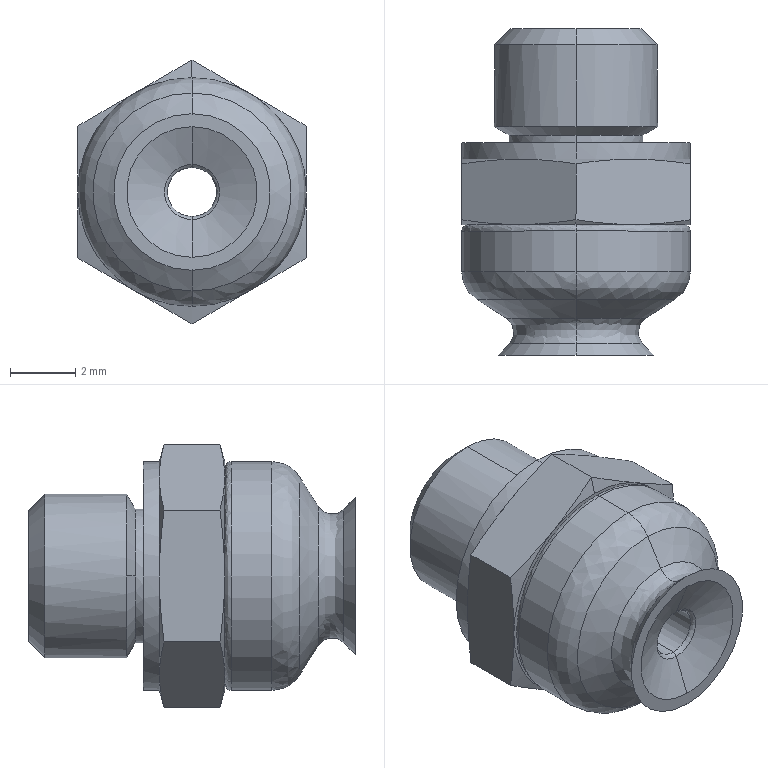Part | SolidWorks | features BaseBody 2 | 2 solids | 55 faces | box 7 x 10 x 8.083 mm | volume 260.959 mm3 | cone 24 | cylinder 12 | plane 11 | spline 8 | commonest cylinder face diameters 1.5 x4 7 x4 4.1 x2 5 x2